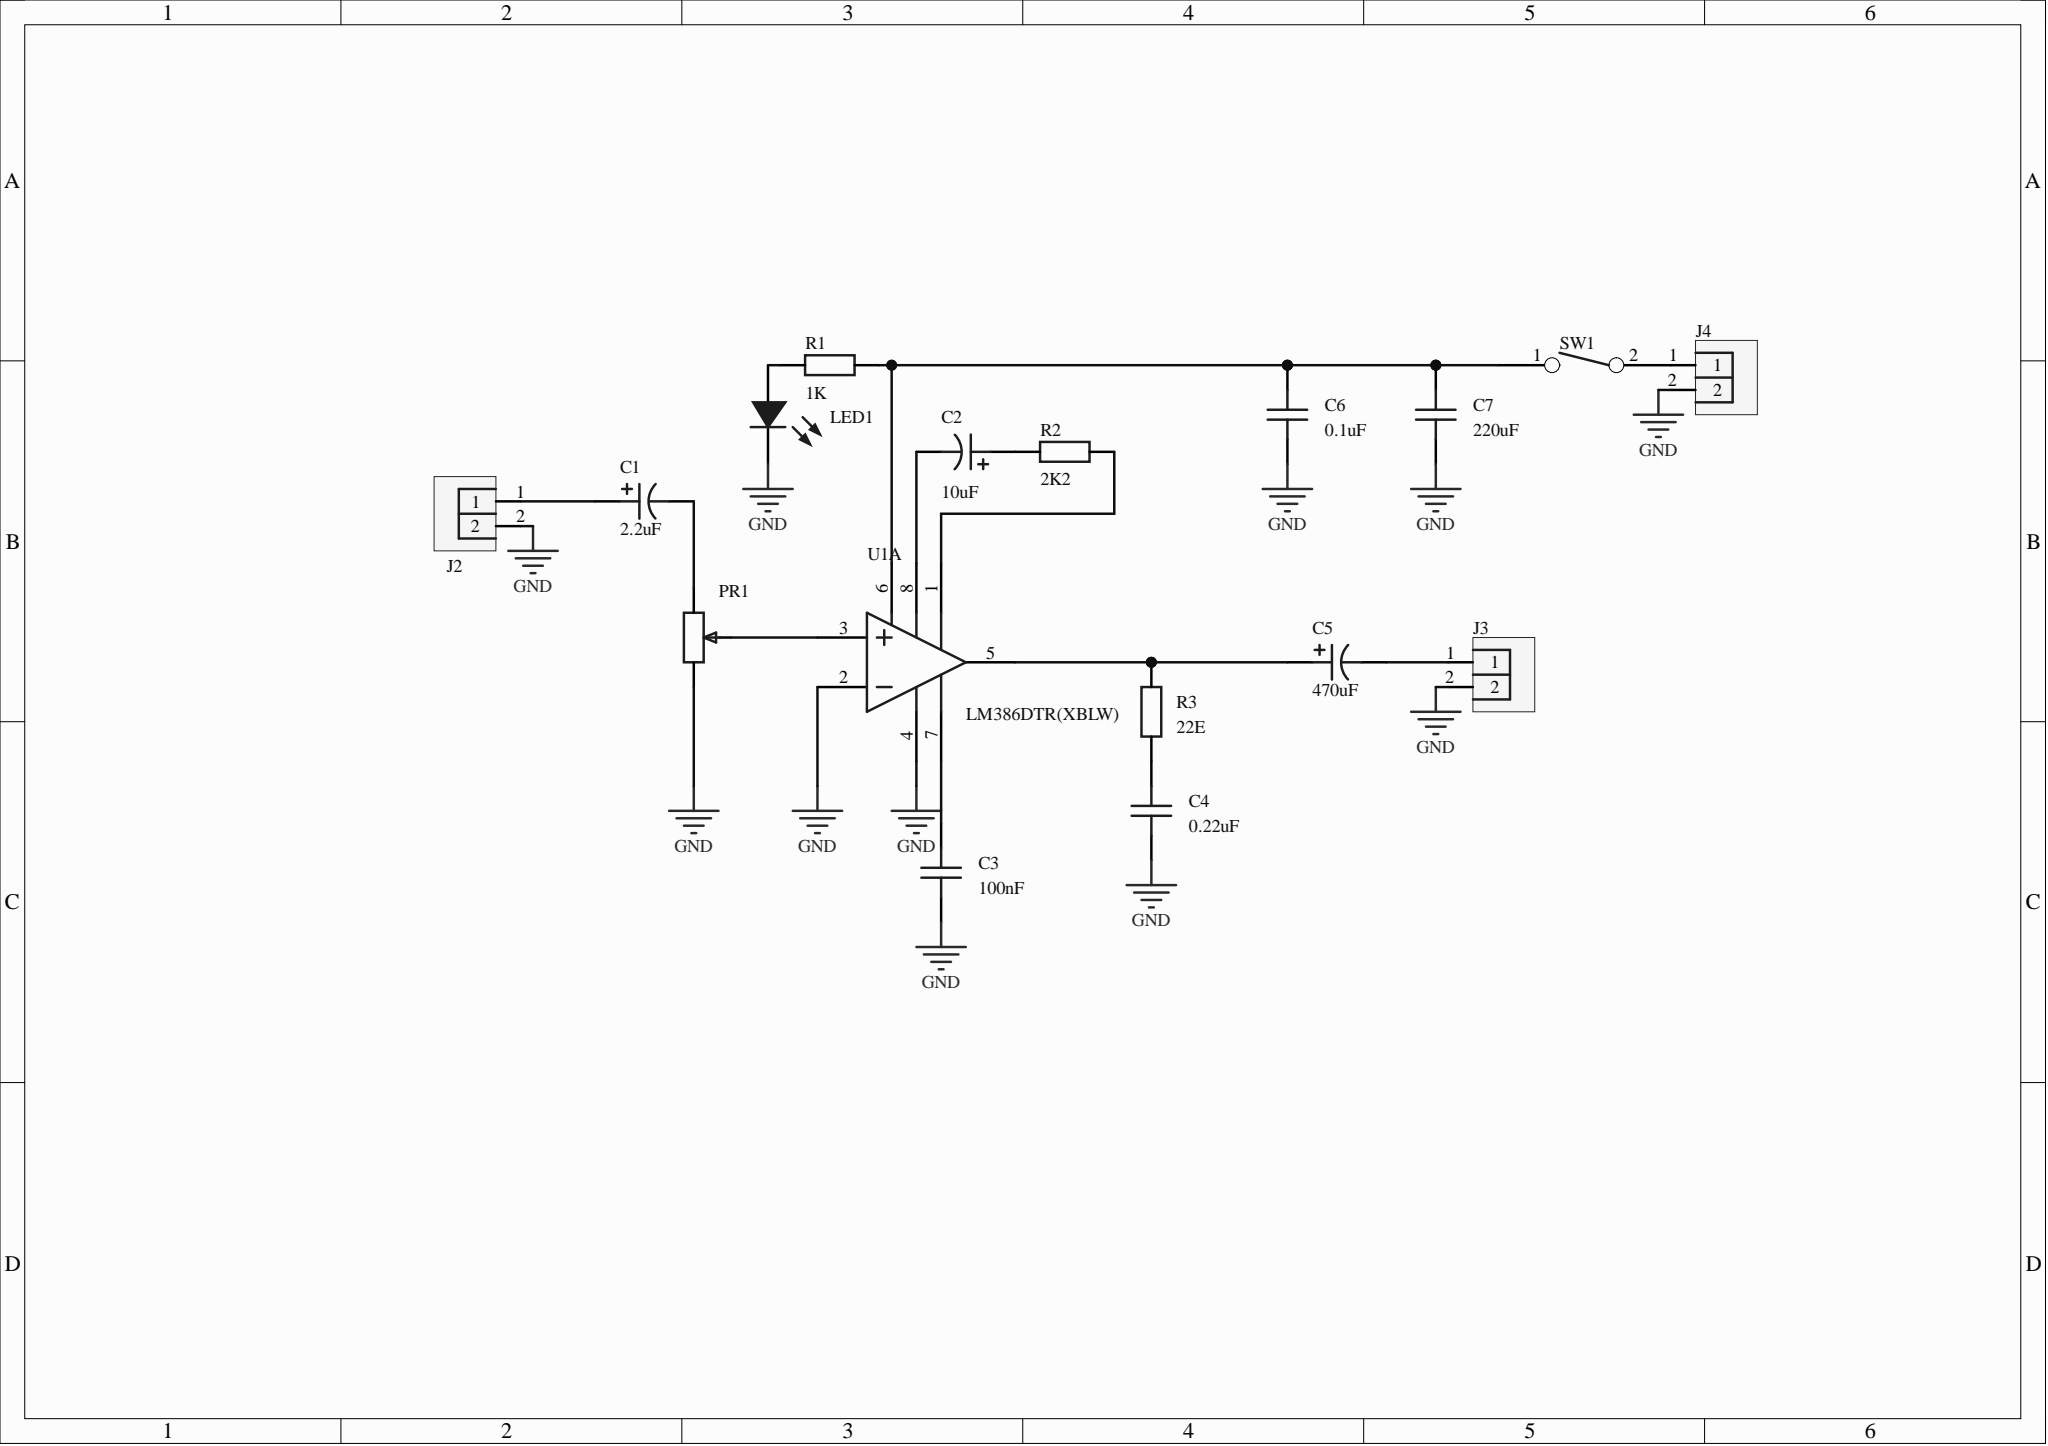Circuit board | Altium Designer | 17 parts | 14 nets
Bill of materials:
Comment,Description,Designator,Footprint,LibRef,Quantity
"2.2uF","","C1","CAP-TH_BD5.0-P2.00-D0.8-FD-10UF50VC110GL","10UF50VC110GL","1"
"10uF","","C2","CAP-TH_BD5.0-P2.00-D0.8-FD-10UF50VC110GL","10UF50VC110GL","1"
"100nF","","C3","C0603","CAP_0603","1"
"0.22uF","","C4","C0603","CAP_0603","1"
"470uF","","C5","CAP-TH_BD5.0-P2.00-D0.8-FD-10UF50VC110GL","10UF50VC110GL","1"
"0.1uF","","C6","C0603","CAP_0603","1"
"220uF","","C7","C0603","CAP_0603","1"
"","","J2, J3, J4","HDR-TH_2P-P2.54-V-M-1","HDR-M_2.54_1x2P","3"
"","","LED1","LED_0603","LED_0603-B","1"
"10kO","","PR1","R_3296","R_3296","1"
"1K","","R1","R0603","Res_0603","1"
"2K2","","R2","R0603","Res_0603","1"
"22E","","R3","R0603","Res_0603","1"
"","","SW1","拨动开关_侧","拨动开关_侧","1"
"LM386DTR(XBLW)","","U1","SOP-8_L4.9-W3.9-P1.27-LS6.0-BL","LM386DTR(XBLW)","1"
Netlist (Protel format):
[
C1
CAP-TH_BD5.0-P2.00-D0.8-FD-10UF50VC110GL
2.2uF



]
[
C2
CAP-TH_BD5.0-P2.00-D0.8-FD-10UF50VC110GL
10uF



]
[
C3
C0603
100nF



]
[
C4
C0603
0.22uF



]
[
C5
CAP-TH_BD5.0-P2.00-D0.8-FD-10UF50VC110GL
470uF



]
[
C6
C0603
0.1uF



]
[
C7
C0603
220uF



]
[
J2
HDR-TH_2P-P2.54-V-M-1




]
[
J3
HDR-TH_2P-P2.54-V-M-1




]
[
J4
HDR-TH_2P-P2.54-V-M-1




]
[
LED1
LED_0603




]
[
PR1
R_3296
10kO



]
[
R1
R0603
1K



]
[
R2
R0603
2K2



]
[
R3
R0603
22E



]
[
SW1
拨动开关_侧




]
[
U1
SOP-8_L4.9-W3.9-P1.27-LS6.0-BL
LM386DTR(XBLW)



]
(
NetR2_2
R2-2
U1-1
)
(
NetPR1_2
PR1-2
U1-3
)
(
NetLED1_2
LED1-2
R1-1
)
(
NetJ4_1
J4-1
SW1-2
)
(
NetC6_2
C6-2
C7-2
R1-2
SW1-1
U1-6
)
(
NetC5_2
C5-2
J3-1
)
(
NetC5_1
C5-1
R3-2
U1-5
)
(
NetC4_2
C4-2
R3-1
)
(
NetC3_2
C3-2
U1-7
)
(
NetC2_2
C2-2
U1-8
)
(
NetC2_1
C2-1
R2-1
)
(
NetC1_2
C1-2
PR1-3
)
(
NetC1_1
C1-1
J2-1
)
(
GND
C3-1
C4-1
C6-1
C7-1
J2-2
J3-2
J4-2
LED1-1
PR1-1
U1-2
U1-4
)